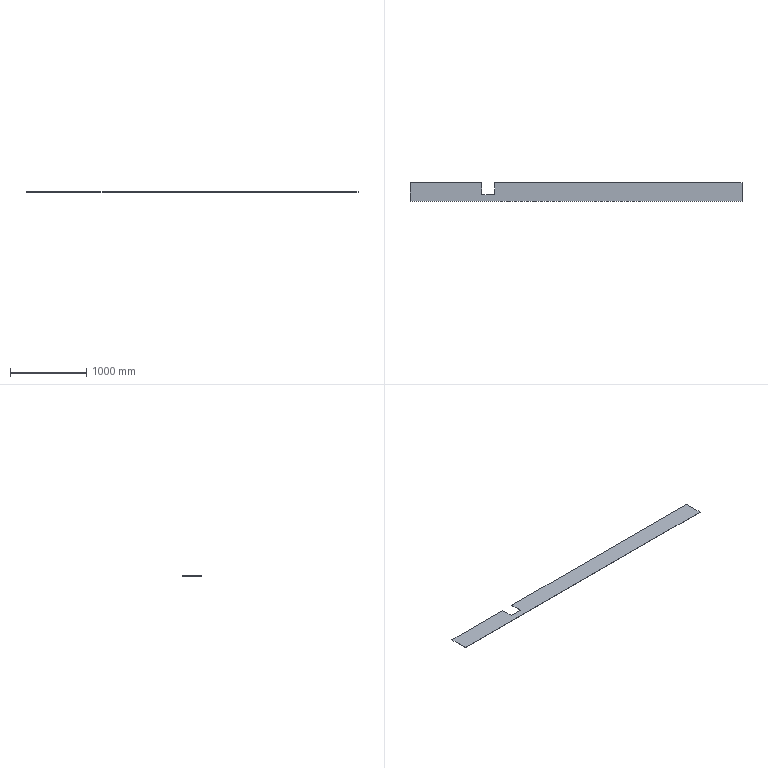Part | STEP file | 休息台花纹Plate 3 | 1 solid | 10 faces | box 4350 x 248 x 3 mm | volume 3156330 mm3 | plane 10
STEP:
#1=CARTESIAN_POINT('',(0.,0.,0.));
#2=DIRECTION('',(0.,0.,1.));
#3=DIRECTION('',(1.,0.,0.));
#4=AXIS2_PLACEMENT_3D('',#1,#2,#3);
#5=CARTESIAN_POINT('',(875.,50.,0.));
#6=VERTEX_POINT('',#5);
#7=CARTESIAN_POINT('',(-2365.,50.,0.));
#8=VERTEX_POINT('',#7);
#9=CARTESIAN_POINT('',(875.,50.,0.));
#10=DIRECTION('',(-1.,0.,0.));
#11=VECTOR('',#10,1.);
#12=LINE('',#9,#11);
#13=CARTESIAN_POINT('',(875.,50.,3.));
#14=DIRECTION('',(0.,-1.,0.));
#15=DIRECTION('',(0.,0.,-1.));
#16=AXIS2_PLACEMENT_3D('',#13,#14,#15);
#17=PLANE('',#16);
#18=CARTESIAN_POINT('',(3.,0.));
#19=DIRECTION('',(0.,-1.));
#20=VECTOR('',#19,1.);
#21=LINE('',#18,#20);
#22=(GEOMETRIC_REPRESENTATION_CONTEXT(2)PARAMETRIC_REPRESENTATION_CONTEXT()REPRESENTATION_CONTEXT('',''));
#23=DEFINITIONAL_REPRESENTATION('',(#21),#22);
#24=PCURVE('',#17,#23);
#25=CARTESIAN_POINT('',(0.,0.,0.));
#26=DIRECTION('',(0.,0.,1.));
#27=DIRECTION('',(1.,0.,0.));
#28=AXIS2_PLACEMENT_3D('',#25,#26,#27);
#29=PLANE('',#28);
#30=CARTESIAN_POINT('',(875.,50.));
#31=DIRECTION('',(-1.,0.));
#32=VECTOR('',#31,1.);
#33=LINE('',#30,#32);
#34=(GEOMETRIC_REPRESENTATION_CONTEXT(2)PARAMETRIC_REPRESENTATION_CONTEXT()REPRESENTATION_CONTEXT('',''));
#35=DEFINITIONAL_REPRESENTATION('',(#33),#34);
#36=PCURVE('',#29,#35);
#37=SURFACE_CURVE('',#12,(#24,#36),.PCURVE_S1.);
#38=EDGE_CURVE('',#6,#8,#37,.T.);
#39=ORIENTED_EDGE('',*,*,#38,.T.);
#40=CARTESIAN_POINT('',(-2365.,50.,3.));
#41=VERTEX_POINT('',#40);
#42=CARTESIAN_POINT('',(-2365.,50.,3.));
#43=DIRECTION('',(0.,0.,-1.));
#44=VECTOR('',#43,1.);
#45=LINE('',#42,#44);
#46=CARTESIAN_POINT('',(0.,-3240.));
#47=DIRECTION('',(1.,0.));
#48=VECTOR('',#47,1.);
#49=LINE('',#46,#48);
#50=(GEOMETRIC_REPRESENTATION_CONTEXT(2)PARAMETRIC_REPRESENTATION_CONTEXT()REPRESENTATION_CONTEXT('',''));
#51=DEFINITIONAL_REPRESENTATION('',(#49),#50);
#52=PCURVE('',#17,#51);
#53=CARTESIAN_POINT('',(-2365.,50.,3.));
#54=DIRECTION('',(1.,0.,0.));
#55=DIRECTION('',(0.,0.,-1.));
#56=AXIS2_PLACEMENT_3D('',#53,#54,#55);
#57=PLANE('',#56);
#58=CARTESIAN_POINT('',(0.,0.));
#59=DIRECTION('',(1.,0.));
#60=VECTOR('',#59,1.);
#61=LINE('',#58,#60);
#62=(GEOMETRIC_REPRESENTATION_CONTEXT(2)PARAMETRIC_REPRESENTATION_CONTEXT()REPRESENTATION_CONTEXT('',''));
#63=DEFINITIONAL_REPRESENTATION('',(#61),#62);
#64=PCURVE('',#57,#63);
#65=SURFACE_CURVE('',#45,(#52,#64),.PCURVE_S1.);
#66=EDGE_CURVE('',#41,#8,#65,.T.);
#67=ORIENTED_EDGE('',*,*,#66,.F.);
#68=CARTESIAN_POINT('',(875.,50.,3.));
#69=VERTEX_POINT('',#68);
#70=CARTESIAN_POINT('',(875.,50.,3.));
#71=DIRECTION('',(-1.,0.,0.));
#72=VECTOR('',#71,1.);
#73=LINE('',#70,#72);
#74=CARTESIAN_POINT('',(0.,0.));
#75=DIRECTION('',(0.,-1.));
#76=VECTOR('',#75,1.);
#77=LINE('',#74,#76);
#78=(GEOMETRIC_REPRESENTATION_CONTEXT(2)PARAMETRIC_REPRESENTATION_CONTEXT()REPRESENTATION_CONTEXT('',''));
#79=DEFINITIONAL_REPRESENTATION('',(#77),#78);
#80=PCURVE('',#17,#79);
#81=CARTESIAN_POINT('',(0.,0.,3.));
#82=DIRECTION('',(0.,0.,1.));
#83=DIRECTION('',(1.,0.,0.));
#84=AXIS2_PLACEMENT_3D('',#81,#82,#83);
#85=PLANE('',#84);
#86=CARTESIAN_POINT('',(875.,50.));
#87=DIRECTION('',(-1.,0.));
#88=VECTOR('',#87,1.);
#89=LINE('',#86,#88);
#90=(GEOMETRIC_REPRESENTATION_CONTEXT(2)PARAMETRIC_REPRESENTATION_CONTEXT()REPRESENTATION_CONTEXT('',''));
#91=DEFINITIONAL_REPRESENTATION('',(#89),#90);
#92=PCURVE('',#85,#91);
#93=SURFACE_CURVE('',#73,(#80,#92),.PCURVE_S1.);
#94=EDGE_CURVE('',#69,#41,#93,.T.);
#95=ORIENTED_EDGE('',*,*,#94,.F.);
#96=CARTESIAN_POINT('',(875.,50.,3.));
#97=DIRECTION('',(0.,0.,-1.));
#98=VECTOR('',#97,1.);
#99=LINE('',#96,#98);
#100=CARTESIAN_POINT('',(0.,0.));
#101=DIRECTION('',(1.,0.));
#102=VECTOR('',#101,1.);
#103=LINE('',#100,#102);
#104=(GEOMETRIC_REPRESENTATION_CONTEXT(2)PARAMETRIC_REPRESENTATION_CONTEXT()REPRESENTATION_CONTEXT('',''));
#105=DEFINITIONAL_REPRESENTATION('',(#103),#104);
#106=PCURVE('',#17,#105);
#107=CARTESIAN_POINT('',(875.,50.,3.));
#108=DIRECTION('',(-1.,0.,0.));
#109=DIRECTION('',(0.,0.,1.));
#110=AXIS2_PLACEMENT_3D('',#107,#108,#109);
#111=PLANE('',#110);
#112=CARTESIAN_POINT('',(0.,0.));
#113=DIRECTION('',(-1.,0.));
#114=VECTOR('',#113,1.);
#115=LINE('',#112,#114);
#116=(GEOMETRIC_REPRESENTATION_CONTEXT(2)PARAMETRIC_REPRESENTATION_CONTEXT()REPRESENTATION_CONTEXT('',''));
#117=DEFINITIONAL_REPRESENTATION('',(#115),#116);
#118=PCURVE('',#111,#117);
#119=SURFACE_CURVE('',#99,(#106,#118),.PCURVE_S1.);
#120=EDGE_CURVE('',#69,#6,#119,.T.);
#121=ORIENTED_EDGE('',*,*,#120,.T.);
#122=EDGE_LOOP('',(#39,#67,#95,#121));
#123=FACE_BOUND('',#122,.T.);
#124=ADVANCED_FACE('',(#123),#17,.F.);
#125=CARTESIAN_POINT('',(-2365.,-107.,0.));
#126=VERTEX_POINT('',#125);
#127=CARTESIAN_POINT('',(-2365.,50.,0.));
#128=DIRECTION('',(0.,-1.,0.));
#129=VECTOR('',#128,1.);
#130=LINE('',#127,#129);
#131=CARTESIAN_POINT('',(3.,0.));
#132=DIRECTION('',(0.,-1.));
#133=VECTOR('',#132,1.);
#134=LINE('',#131,#133);
#135=(GEOMETRIC_REPRESENTATION_CONTEXT(2)PARAMETRIC_REPRESENTATION_CONTEXT()REPRESENTATION_CONTEXT('',''));
#136=DEFINITIONAL_REPRESENTATION('',(#134),#135);
#137=PCURVE('',#57,#136);
#138=CARTESIAN_POINT('',(-2365.,50.));
#139=DIRECTION('',(0.,-1.));
#140=VECTOR('',#139,1.);
#141=LINE('',#138,#140);
#142=(GEOMETRIC_REPRESENTATION_CONTEXT(2)PARAMETRIC_REPRESENTATION_CONTEXT()REPRESENTATION_CONTEXT('',''));
#143=DEFINITIONAL_REPRESENTATION('',(#141),#142);
#144=PCURVE('',#29,#143);
#145=SURFACE_CURVE('',#130,(#137,#144),.PCURVE_S1.);
#146=EDGE_CURVE('',#8,#126,#145,.T.);
#147=ORIENTED_EDGE('',*,*,#146,.T.);
#148=CARTESIAN_POINT('',(-2365.,-107.,3.));
#149=VERTEX_POINT('',#148);
#150=CARTESIAN_POINT('',(-2365.,-107.,3.));
#151=DIRECTION('',(0.,0.,-1.));
#152=VECTOR('',#151,1.);
#153=LINE('',#150,#152);
#154=CARTESIAN_POINT('',(0.,-157.));
#155=DIRECTION('',(1.,0.));
#156=VECTOR('',#155,1.);
#157=LINE('',#154,#156);
#158=(GEOMETRIC_REPRESENTATION_CONTEXT(2)PARAMETRIC_REPRESENTATION_CONTEXT()REPRESENTATION_CONTEXT('',''));
#159=DEFINITIONAL_REPRESENTATION('',(#157),#158);
#160=PCURVE('',#57,#159);
#161=CARTESIAN_POINT('',(-2365.,-107.,3.));
#162=DIRECTION('',(0.,-1.,0.));
#163=DIRECTION('',(1.,0.,0.));
#164=AXIS2_PLACEMENT_3D('',#161,#162,#163);
#165=PLANE('',#164);
#166=CARTESIAN_POINT('',(0.,0.));
#167=DIRECTION('',(0.,-1.));
#168=VECTOR('',#167,1.);
#169=LINE('',#166,#168);
#170=(GEOMETRIC_REPRESENTATION_CONTEXT(2)PARAMETRIC_REPRESENTATION_CONTEXT()REPRESENTATION_CONTEXT('',''));
#171=DEFINITIONAL_REPRESENTATION('',(#169),#170);
#172=PCURVE('',#165,#171);
#173=SURFACE_CURVE('',#153,(#160,#172),.PCURVE_S1.);
#174=EDGE_CURVE('',#149,#126,#173,.T.);
#175=ORIENTED_EDGE('',*,*,#174,.F.);
#176=CARTESIAN_POINT('',(-2365.,50.,3.));
#177=DIRECTION('',(0.,-1.,0.));
#178=VECTOR('',#177,1.);
#179=LINE('',#176,#178);
#180=CARTESIAN_POINT('',(0.,0.));
#181=DIRECTION('',(0.,-1.));
#182=VECTOR('',#181,1.);
#183=LINE('',#180,#182);
#184=(GEOMETRIC_REPRESENTATION_CONTEXT(2)PARAMETRIC_REPRESENTATION_CONTEXT()REPRESENTATION_CONTEXT('',''));
#185=DEFINITIONAL_REPRESENTATION('',(#183),#184);
#186=PCURVE('',#57,#185);
#187=CARTESIAN_POINT('',(-2365.,50.));
#188=DIRECTION('',(0.,-1.));
#189=VECTOR('',#188,1.);
#190=LINE('',#187,#189);
#191=(GEOMETRIC_REPRESENTATION_CONTEXT(2)PARAMETRIC_REPRESENTATION_CONTEXT()REPRESENTATION_CONTEXT('',''));
#192=DEFINITIONAL_REPRESENTATION('',(#190),#191);
#193=PCURVE('',#85,#192);
#194=SURFACE_CURVE('',#179,(#186,#193),.PCURVE_S1.);
#195=EDGE_CURVE('',#41,#149,#194,.T.);
#196=ORIENTED_EDGE('',*,*,#195,.F.);
#197=ORIENTED_EDGE('',*,*,#66,.T.);
#198=EDGE_LOOP('',(#147,#175,#196,#197));
#199=FACE_BOUND('',#198,.T.);
#200=ADVANCED_FACE('',(#199),#57,.F.);
#201=CARTESIAN_POINT('',(-2535.,-107.,0.));
#202=VERTEX_POINT('',#201);
#203=CARTESIAN_POINT('',(-2365.,-107.,0.));
#204=DIRECTION('',(-1.,0.,0.));
#205=VECTOR('',#204,1.);
#206=LINE('',#203,#205);
#207=CARTESIAN_POINT('',(0.,-3.));
#208=DIRECTION('',(-1.,0.));
#209=VECTOR('',#208,1.);
#210=LINE('',#207,#209);
#211=(GEOMETRIC_REPRESENTATION_CONTEXT(2)PARAMETRIC_REPRESENTATION_CONTEXT()REPRESENTATION_CONTEXT('',''));
#212=DEFINITIONAL_REPRESENTATION('',(#210),#211);
#213=PCURVE('',#165,#212);
#214=CARTESIAN_POINT('',(-2365.,-107.));
#215=DIRECTION('',(-1.,0.));
#216=VECTOR('',#215,1.);
#217=LINE('',#214,#216);
#218=(GEOMETRIC_REPRESENTATION_CONTEXT(2)PARAMETRIC_REPRESENTATION_CONTEXT()REPRESENTATION_CONTEXT('',''));
#219=DEFINITIONAL_REPRESENTATION('',(#217),#218);
#220=PCURVE('',#29,#219);
#221=SURFACE_CURVE('',#206,(#213,#220),.PCURVE_S1.);
#222=EDGE_CURVE('',#126,#202,#221,.T.);
#223=ORIENTED_EDGE('',*,*,#222,.T.);
#224=CARTESIAN_POINT('',(-2535.,-107.,3.));
#225=VERTEX_POINT('',#224);
#226=CARTESIAN_POINT('',(-2535.,-107.,3.));
#227=DIRECTION('',(0.,0.,-1.));
#228=VECTOR('',#227,1.);
#229=LINE('',#226,#228);
#230=CARTESIAN_POINT('',(-170.,0.));
#231=DIRECTION('',(0.,-1.));
#232=VECTOR('',#231,1.);
#233=LINE('',#230,#232);
#234=(GEOMETRIC_REPRESENTATION_CONTEXT(2)PARAMETRIC_REPRESENTATION_CONTEXT()REPRESENTATION_CONTEXT('',''));
#235=DEFINITIONAL_REPRESENTATION('',(#233),#234);
#236=PCURVE('',#165,#235);
#237=CARTESIAN_POINT('',(-2535.,50.,3.));
#238=DIRECTION('',(-1.,0.,0.));
#239=DIRECTION('',(0.,0.,1.));
#240=AXIS2_PLACEMENT_3D('',#237,#238,#239);
#241=PLANE('',#240);
#242=CARTESIAN_POINT('',(0.,-157.));
#243=DIRECTION('',(-1.,0.));
#244=VECTOR('',#243,1.);
#245=LINE('',#242,#244);
#246=(GEOMETRIC_REPRESENTATION_CONTEXT(2)PARAMETRIC_REPRESENTATION_CONTEXT()REPRESENTATION_CONTEXT('',''));
#247=DEFINITIONAL_REPRESENTATION('',(#245),#246);
#248=PCURVE('',#241,#247);
#249=SURFACE_CURVE('',#229,(#236,#248),.PCURVE_S1.);
#250=EDGE_CURVE('',#225,#202,#249,.T.);
#251=ORIENTED_EDGE('',*,*,#250,.F.);
#252=CARTESIAN_POINT('',(-2365.,-107.,3.));
#253=DIRECTION('',(-1.,0.,0.));
#254=VECTOR('',#253,1.);
#255=LINE('',#252,#254);
#256=CARTESIAN_POINT('',(0.,0.));
#257=DIRECTION('',(-1.,0.));
#258=VECTOR('',#257,1.);
#259=LINE('',#256,#258);
#260=(GEOMETRIC_REPRESENTATION_CONTEXT(2)PARAMETRIC_REPRESENTATION_CONTEXT()REPRESENTATION_CONTEXT('',''));
#261=DEFINITIONAL_REPRESENTATION('',(#259),#260);
#262=PCURVE('',#165,#261);
#263=CARTESIAN_POINT('',(-2365.,-107.));
#264=DIRECTION('',(-1.,0.));
#265=VECTOR('',#264,1.);
#266=LINE('',#263,#265);
#267=(GEOMETRIC_REPRESENTATION_CONTEXT(2)PARAMETRIC_REPRESENTATION_CONTEXT()REPRESENTATION_CONTEXT('',''));
#268=DEFINITIONAL_REPRESENTATION('',(#266),#267);
#269=PCURVE('',#85,#268);
#270=SURFACE_CURVE('',#255,(#262,#269),.PCURVE_S1.);
#271=EDGE_CURVE('',#149,#225,#270,.T.);
#272=ORIENTED_EDGE('',*,*,#271,.F.);
#273=ORIENTED_EDGE('',*,*,#174,.T.);
#274=EDGE_LOOP('',(#223,#251,#272,#273));
#275=FACE_BOUND('',#274,.T.);
#276=ADVANCED_FACE('',(#275),#165,.F.);
#277=CARTESIAN_POINT('',(-2535.,50.,0.));
#278=VERTEX_POINT('',#277);
#279=CARTESIAN_POINT('',(-2535.,50.,0.));
#280=DIRECTION('',(0.,1.,0.));
#281=VECTOR('',#280,1.);
#282=LINE('',#279,#281);
#283=CARTESIAN_POINT('',(-3.,0.));
#284=DIRECTION('',(0.,1.));
#285=VECTOR('',#284,1.);
#286=LINE('',#283,#285);
#287=(GEOMETRIC_REPRESENTATION_CONTEXT(2)PARAMETRIC_REPRESENTATION_CONTEXT()REPRESENTATION_CONTEXT('',''));
#288=DEFINITIONAL_REPRESENTATION('',(#286),#287);
#289=PCURVE('',#241,#288);
#290=CARTESIAN_POINT('',(-2535.,50.));
#291=DIRECTION('',(0.,1.));
#292=VECTOR('',#291,1.);
#293=LINE('',#290,#292);
#294=(GEOMETRIC_REPRESENTATION_CONTEXT(2)PARAMETRIC_REPRESENTATION_CONTEXT()REPRESENTATION_CONTEXT('',''));
#295=DEFINITIONAL_REPRESENTATION('',(#293),#294);
#296=PCURVE('',#29,#295);
#297=SURFACE_CURVE('',#282,(#289,#296),.PCURVE_S1.);
#298=EDGE_CURVE('',#202,#278,#297,.T.);
#299=ORIENTED_EDGE('',*,*,#298,.T.);
#300=CARTESIAN_POINT('',(-2535.,50.,3.));
#301=VERTEX_POINT('',#300);
#302=CARTESIAN_POINT('',(-2535.,50.,3.));
#303=DIRECTION('',(0.,0.,-1.));
#304=VECTOR('',#303,1.);
#305=LINE('',#302,#304);
#306=CARTESIAN_POINT('',(0.,0.));
#307=DIRECTION('',(-1.,0.));
#308=VECTOR('',#307,1.);
#309=LINE('',#306,#308);
#310=(GEOMETRIC_REPRESENTATION_CONTEXT(2)PARAMETRIC_REPRESENTATION_CONTEXT()REPRESENTATION_CONTEXT('',''));
#311=DEFINITIONAL_REPRESENTATION('',(#309),#310);
#312=PCURVE('',#241,#311);
#313=CARTESIAN_POINT('',(-2535.,50.,3.));
#314=DIRECTION('',(0.,-1.,0.));
#315=DIRECTION('',(1.,0.,0.));
#316=AXIS2_PLACEMENT_3D('',#313,#314,#315);
#317=PLANE('',#316);
#318=CARTESIAN_POINT('',(0.,0.));
#319=DIRECTION('',(0.,-1.));
#320=VECTOR('',#319,1.);
#321=LINE('',#318,#320);
#322=(GEOMETRIC_REPRESENTATION_CONTEXT(2)PARAMETRIC_REPRESENTATION_CONTEXT()REPRESENTATION_CONTEXT('',''));
#323=DEFINITIONAL_REPRESENTATION('',(#321),#322);
#324=PCURVE('',#317,#323);
#325=SURFACE_CURVE('',#305,(#312,#324),.PCURVE_S1.);
#326=EDGE_CURVE('',#301,#278,#325,.T.);
#327=ORIENTED_EDGE('',*,*,#326,.F.);
#328=CARTESIAN_POINT('',(-2535.,50.,3.));
#329=DIRECTION('',(0.,1.,0.));
#330=VECTOR('',#329,1.);
#331=LINE('',#328,#330);
#332=CARTESIAN_POINT('',(0.,0.));
#333=DIRECTION('',(0.,1.));
#334=VECTOR('',#333,1.);
#335=LINE('',#332,#334);
#336=(GEOMETRIC_REPRESENTATION_CONTEXT(2)PARAMETRIC_REPRESENTATION_CONTEXT()REPRESENTATION_CONTEXT('',''));
#337=DEFINITIONAL_REPRESENTATION('',(#335),#336);
#338=PCURVE('',#241,#337);
#339=CARTESIAN_POINT('',(-2535.,50.));
#340=DIRECTION('',(0.,1.));
#341=VECTOR('',#340,1.);
#342=LINE('',#339,#341);
#343=(GEOMETRIC_REPRESENTATION_CONTEXT(2)PARAMETRIC_REPRESENTATION_CONTEXT()REPRESENTATION_CONTEXT('',''));
#344=DEFINITIONAL_REPRESENTATION('',(#342),#343);
#345=PCURVE('',#85,#344);
#346=SURFACE_CURVE('',#331,(#338,#345),.PCURVE_S1.);
#347=EDGE_CURVE('',#225,#301,#346,.T.);
#348=ORIENTED_EDGE('',*,*,#347,.F.);
#349=ORIENTED_EDGE('',*,*,#250,.T.);
#350=EDGE_LOOP('',(#299,#327,#348,#349));
#351=FACE_BOUND('',#350,.T.);
#352=ADVANCED_FACE('',(#351),#241,.F.);
#353=CARTESIAN_POINT('',(-3475.,50.,0.));
#354=VERTEX_POINT('',#353);
#355=CARTESIAN_POINT('',(-2535.,50.,0.));
#356=DIRECTION('',(-1.,0.,0.));
#357=VECTOR('',#356,1.);
#358=LINE('',#355,#357);
#359=CARTESIAN_POINT('',(0.,-3.));
#360=DIRECTION('',(-1.,0.));
#361=VECTOR('',#360,1.);
#362=LINE('',#359,#361);
#363=(GEOMETRIC_REPRESENTATION_CONTEXT(2)PARAMETRIC_REPRESENTATION_CONTEXT()REPRESENTATION_CONTEXT('',''));
#364=DEFINITIONAL_REPRESENTATION('',(#362),#363);
#365=PCURVE('',#317,#364);
#366=CARTESIAN_POINT('',(-2535.,50.));
#367=DIRECTION('',(-1.,0.));
#368=VECTOR('',#367,1.);
#369=LINE('',#366,#368);
#370=(GEOMETRIC_REPRESENTATION_CONTEXT(2)PARAMETRIC_REPRESENTATION_CONTEXT()REPRESENTATION_CONTEXT('',''));
#371=DEFINITIONAL_REPRESENTATION('',(#369),#370);
#372=PCURVE('',#29,#371);
#373=SURFACE_CURVE('',#358,(#365,#372),.PCURVE_S1.);
#374=EDGE_CURVE('',#278,#354,#373,.T.);
#375=ORIENTED_EDGE('',*,*,#374,.T.);
#376=CARTESIAN_POINT('',(-3475.,50.,3.));
#377=VERTEX_POINT('',#376);
#378=CARTESIAN_POINT('',(-3475.,50.,3.));
#379=DIRECTION('',(0.,0.,-1.));
#380=VECTOR('',#379,1.);
#381=LINE('',#378,#380);
#382=CARTESIAN_POINT('',(-940.,0.));
#383=DIRECTION('',(0.,-1.));
#384=VECTOR('',#383,1.);
#385=LINE('',#382,#384);
#386=(GEOMETRIC_REPRESENTATION_CONTEXT(2)PARAMETRIC_REPRESENTATION_CONTEXT()REPRESENTATION_CONTEXT('',''));
#387=DEFINITIONAL_REPRESENTATION('',(#385),#386);
#388=PCURVE('',#317,#387);
#389=CARTESIAN_POINT('',(-3475.,50.,3.));
#390=DIRECTION('',(1.,0.,0.));
#391=DIRECTION('',(0.,0.,-1.));
#392=AXIS2_PLACEMENT_3D('',#389,#390,#391);
#393=PLANE('',#392);
#394=CARTESIAN_POINT('',(0.,0.));
#395=DIRECTION('',(1.,0.));
#396=VECTOR('',#395,1.);
#397=LINE('',#394,#396);
#398=(GEOMETRIC_REPRESENTATION_CONTEXT(2)PARAMETRIC_REPRESENTATION_CONTEXT()REPRESENTATION_CONTEXT('',''));
#399=DEFINITIONAL_REPRESENTATION('',(#397),#398);
#400=PCURVE('',#393,#399);
#401=SURFACE_CURVE('',#381,(#388,#400),.PCURVE_S1.);
#402=EDGE_CURVE('',#377,#354,#401,.T.);
#403=ORIENTED_EDGE('',*,*,#402,.F.);
#404=CARTESIAN_POINT('',(-2535.,50.,3.));
#405=DIRECTION('',(-1.,0.,0.));
#406=VECTOR('',#405,1.);
#407=LINE('',#404,#406);
#408=CARTESIAN_POINT('',(0.,0.));
#409=DIRECTION('',(-1.,0.));
#410=VECTOR('',#409,1.);
#411=LINE('',#408,#410);
#412=(GEOMETRIC_REPRESENTATION_CONTEXT(2)PARAMETRIC_REPRESENTATION_CONTEXT()REPRESENTATION_CONTEXT('',''));
#413=DEFINITIONAL_REPRESENTATION('',(#411),#412);
#414=PCURVE('',#317,#413);
#415=CARTESIAN_POINT('',(-2535.,50.));
#416=DIRECTION('',(-1.,0.));
#417=VECTOR('',#416,1.);
#418=LINE('',#415,#417);
#419=(GEOMETRIC_REPRESENTATION_CONTEXT(2)PARAMETRIC_REPRESENTATION_CONTEXT()REPRESENTATION_CONTEXT('',''));
#420=DEFINITIONAL_REPRESENTATION('',(#418),#419);
#421=PCURVE('',#85,#420);
#422=SURFACE_CURVE('',#407,(#414,#421),.PCURVE_S1.);
#423=EDGE_CURVE('',#301,#377,#422,.T.);
#424=ORIENTED_EDGE('',*,*,#423,.F.);
#425=ORIENTED_EDGE('',*,*,#326,.T.);
#426=EDGE_LOOP('',(#375,#403,#424,#425));
#427=FACE_BOUND('',#426,.T.);
#428=ADVANCED_FACE('',(#427),#317,.F.);
#429=CARTESIAN_POINT('',(-3475.,-198.,0.));
#430=VERTEX_POINT('',#429);
#431=CARTESIAN_POINT('',(-3475.,50.,0.));
#432=DIRECTION('',(0.,-1.,0.));
#433=VECTOR('',#432,1.);
#434=LINE('',#431,#433);
#435=CARTESIAN_POINT('',(3.,0.));
#436=DIRECTION('',(0.,-1.));
#437=VECTOR('',#436,1.);
#438=LINE('',#435,#437);
#439=(GEOMETRIC_REPRESENTATION_CONTEXT(2)PARAMETRIC_REPRESENTATION_CONTEXT()REPRESENTATION_CONTEXT('',''));
#440=DEFINITIONAL_REPRESENTATION('',(#438),#439);
#441=PCURVE('',#393,#440);
#442=CARTESIAN_POINT('',(-3475.,50.));
#443=DIRECTION('',(0.,-1.));
#444=VECTOR('',#443,1.);
#445=LINE('',#442,#444);
#446=(GEOMETRIC_REPRESENTATION_CONTEXT(2)PARAMETRIC_REPRESENTATION_CONTEXT()REPRESENTATION_CONTEXT('',''));
#447=DEFINITIONAL_REPRESENTATION('',(#445),#446);
#448=PCURVE('',#29,#447);
#449=SURFACE_CURVE('',#434,(#441,#448),.PCURVE_S1.);
#450=EDGE_CURVE('',#354,#430,#449,.T.);
#451=ORIENTED_EDGE('',*,*,#450,.T.);
#452=CARTESIAN_POINT('',(-3475.,-198.,3.));
#453=VERTEX_POINT('',#452);
#454=CARTESIAN_POINT('',(-3475.,-198.,3.));
#455=DIRECTION('',(0.,0.,-1.));
#456=VECTOR('',#455,1.);
#457=LINE('',#454,#456);
#458=CARTESIAN_POINT('',(0.,-248.));
#459=DIRECTION('',(1.,0.));
#460=VECTOR('',#459,1.);
#461=LINE('',#458,#460);
#462=(GEOMETRIC_REPRESENTATION_CONTEXT(2)PARAMETRIC_REPRESENTATION_CONTEXT()REPRESENTATION_CONTEXT('',''));
#463=DEFINITIONAL_REPRESENTATION('',(#461),#462);
#464=PCURVE('',#393,#463);
#465=CARTESIAN_POINT('',(875.,-198.,3.));
#466=DIRECTION('',(0.,1.,0.));
#467=DIRECTION('',(-1.,0.,0.));
#468=AXIS2_PLACEMENT_3D('',#465,#466,#467);
#469=PLANE('',#468);
#470=CARTESIAN_POINT('',(4350.,0.));
#471=DIRECTION('',(0.,-1.));
#472=VECTOR('',#471,1.);
#473=LINE('',#470,#472);
#474=(GEOMETRIC_REPRESENTATION_CONTEXT(2)PARAMETRIC_REPRESENTATION_CONTEXT()REPRESENTATION_CONTEXT('',''));
#475=DEFINITIONAL_REPRESENTATION('',(#473),#474);
#476=PCURVE('',#469,#475);
#477=SURFACE_CURVE('',#457,(#464,#476),.PCURVE_S1.);
#478=EDGE_CURVE('',#453,#430,#477,.T.);
#479=ORIENTED_EDGE('',*,*,#478,.F.);
#480=CARTESIAN_POINT('',(-3475.,50.,3.));
#481=DIRECTION('',(0.,-1.,0.));
#482=VECTOR('',#481,1.);
#483=LINE('',#480,#482);
#484=CARTESIAN_POINT('',(0.,0.));
#485=DIRECTION('',(0.,-1.));
#486=VECTOR('',#485,1.);
#487=LINE('',#484,#486);
#488=(GEOMETRIC_REPRESENTATION_CONTEXT(2)PARAMETRIC_REPRESENTATION_CONTEXT()REPRESENTATION_CONTEXT('',''));
#489=DEFINITIONAL_REPRESENTATION('',(#487),#488);
#490=PCURVE('',#393,#489);
#491=CARTESIAN_POINT('',(-3475.,50.));
#492=DIRECTION('',(0.,-1.));
#493=VECTOR('',#492,1.);
#494=LINE('',#491,#493);
#495=(GEOMETRIC_REPRESENTATION_CONTEXT(2)PARAMETRIC_REPRESENTATION_CONTEXT()REPRESENTATION_CONTEXT('',''));
#496=DEFINITIONAL_REPRESENTATION('',(#494),#495);
#497=PCURVE('',#85,#496);
#498=SURFACE_CURVE('',#483,(#490,#497),.PCURVE_S1.);
#499=EDGE_CURVE('',#377,#453,#498,.T.);
#500=ORIENTED_EDGE('',*,*,#499,.F.);
#501=ORIENTED_EDGE('',*,*,#402,.T.);
#502=EDGE_LOOP('',(#451,#479,#500,#501));
#503=FACE_BOUND('',#502,.T.);
#504=ADVANCED_FACE('',(#503),#393,.F.);
#505=CARTESIAN_POINT('',(875.,-198.,0.));
#506=VERTEX_POINT('',#505);
#507=CARTESIAN_POINT('',(875.,-198.,0.));
#508=DIRECTION('',(1.,0.,0.));
#509=VECTOR('',#508,1.);
#510=LINE('',#507,#509);
#511=CARTESIAN_POINT('',(0.,-3.));
#512=DIRECTION('',(-1.,0.));
#513=VECTOR('',#512,1.);
#514=LINE('',#511,#513);
#515=(GEOMETRIC_REPRESENTATION_CONTEXT(2)PARAMETRIC_REPRESENTATION_CONTEXT()REPRESENTATION_CONTEXT('',''));
#516=DEFINITIONAL_REPRESENTATION('',(#514),#515);
#517=PCURVE('',#469,#516);
#518=CARTESIAN_POINT('',(875.,-198.));
#519=DIRECTION('',(1.,0.));
#520=VECTOR('',#519,1.);
#521=LINE('',#518,#520);
#522=(GEOMETRIC_REPRESENTATION_CONTEXT(2)PARAMETRIC_REPRESENTATION_CONTEXT()REPRESENTATION_CONTEXT('',''));
#523=DEFINITIONAL_REPRESENTATION('',(#521),#522);
#524=PCURVE('',#29,#523);
#525=SURFACE_CURVE('',#510,(#517,#524),.PCURVE_S1.);
#526=EDGE_CURVE('',#430,#506,#525,.T.);
#527=ORIENTED_EDGE('',*,*,#526,.T.);
#528=CARTESIAN_POINT('',(875.,-198.,3.));
#529=VERTEX_POINT('',#528);
#530=CARTESIAN_POINT('',(875.,-198.,3.));
#531=DIRECTION('',(0.,0.,-1.));
#532=VECTOR('',#531,1.);
#533=LINE('',#530,#532);
#534=CARTESIAN_POINT('',(0.,0.));
#535=DIRECTION('',(0.,-1.));
#536=VECTOR('',#535,1.);
#537=LINE('',#534,#536);
#538=(GEOMETRIC_REPRESENTATION_CONTEXT(2)PARAMETRIC_REPRESENTATION_CONTEXT()REPRESENTATION_CONTEXT('',''));
#539=DEFINITIONAL_REPRESENTATION('',(#537),#538);
#540=PCURVE('',#469,#539);
#541=CARTESIAN_POINT('',(0.,-248.));
#542=DIRECTION('',(-1.,0.));
#543=VECTOR('',#542,1.);
#544=LINE('',#541,#543);
#545=(GEOMETRIC_REPRESENTATION_CONTEXT(2)PARAMETRIC_REPRESENTATION_CONTEXT()REPRESENTATION_CONTEXT('',''));
#546=DEFINITIONAL_REPRESENTATION('',(#544),#545);
#547=PCURVE('',#111,#546);
#548=SURFACE_CURVE('',#533,(#540,#547),.PCURVE_S1.);
#549=EDGE_CURVE('',#529,#506,#548,.T.);
#550=ORIENTED_EDGE('',*,*,#549,.F.);
#551=CARTESIAN_POINT('',(875.,-198.,3.));
#552=DIRECTION('',(1.,0.,0.));
#553=VECTOR('',#552,1.);
#554=LINE('',#551,#553);
#555=CARTESIAN_POINT('',(0.,0.));
#556=DIRECTION('',(-1.,0.));
#557=VECTOR('',#556,1.);
#558=LINE('',#555,#557);
#559=(GEOMETRIC_REPRESENTATION_CONTEXT(2)PARAMETRIC_REPRESENTATION_CONTEXT()REPRESENTATION_CONTEXT('',''));
#560=DEFINITIONAL_REPRESENTATION('',(#558),#559);
#561=PCURVE('',#469,#560);
#562=CARTESIAN_POINT('',(875.,-198.));
#563=DIRECTION('',(1.,0.));
#564=VECTOR('',#563,1.);
#565=LINE('',#562,#564);
#566=(GEOMETRIC_REPRESENTATION_CONTEXT(2)PARAMETRIC_REPRESENTATION_CONTEXT()REPRESENTATION_CONTEXT('',''));
#567=DEFINITIONAL_REPRESENTATION('',(#565),#566);
#568=PCURVE('',#85,#567);
#569=SURFACE_CURVE('',#554,(#561,#568),.PCURVE_S1.);
#570=EDGE_CURVE('',#453,#529,#569,.T.);
#571=ORIENTED_EDGE('',*,*,#570,.F.);
#572=ORIENTED_EDGE('',*,*,#478,.T.);
#573=EDGE_LOOP('',(#527,#550,#571,#572));
#574=FACE_BOUND('',#573,.T.);
#575=ADVANCED_FACE('',(#574),#469,.F.);
#576=CARTESIAN_POINT('',(875.,50.,0.));
#577=DIRECTION('',(0.,1.,0.));
#578=VECTOR('',#577,1.);
#579=LINE('',#576,#578);
#580=CARTESIAN_POINT('',(-3.,0.));
#581=DIRECTION('',(0.,1.));
#582=VECTOR('',#581,1.);
#583=LINE('',#580,#582);
#584=(GEOMETRIC_REPRESENTATION_CONTEXT(2)PARAMETRIC_REPRESENTATION_CONTEXT()REPRESENTATION_CONTEXT('',''));
#585=DEFINITIONAL_REPRESENTATION('',(#583),#584);
#586=PCURVE('',#111,#585);
#587=CARTESIAN_POINT('',(875.,50.));
#588=DIRECTION('',(0.,1.));
#589=VECTOR('',#588,1.);
#590=LINE('',#587,#589);
#591=(GEOMETRIC_REPRESENTATION_CONTEXT(2)PARAMETRIC_REPRESENTATION_CONTEXT()REPRESENTATION_CONTEXT('',''));
#592=DEFINITIONAL_REPRESENTATION('',(#590),#591);
#593=PCURVE('',#29,#592);
#594=SURFACE_CURVE('',#579,(#586,#593),.PCURVE_S1.);
#595=EDGE_CURVE('',#506,#6,#594,.T.);
#596=ORIENTED_EDGE('',*,*,#595,.T.);
#597=ORIENTED_EDGE('',*,*,#120,.F.);
#598=CARTESIAN_POINT('',(875.,50.,3.));
#599=DIRECTION('',(0.,1.,0.));
#600=VECTOR('',#599,1.);
#601=LINE('',#598,#600);
#602=CARTESIAN_POINT('',(0.,0.));
#603=DIRECTION('',(0.,1.));
#604=VECTOR('',#603,1.);
#605=LINE('',#602,#604);
#606=(GEOMETRIC_REPRESENTATION_CONTEXT(2)PARAMETRIC_REPRESENTATION_CONTEXT()REPRESENTATION_CONTEXT('',''));
#607=DEFINITIONAL_REPRESENTATION('',(#605),#606);
#608=PCURVE('',#111,#607);
#609=CARTESIAN_POINT('',(875.,50.));
#610=DIRECTION('',(0.,1.));
#611=VECTOR('',#610,1.);
#612=LINE('',#609,#611);
#613=(GEOMETRIC_REPRESENTATION_CONTEXT(2)PARAMETRIC_REPRESENTATION_CONTEXT()REPRESENTATION_CONTEXT('',''));
#614=DEFINITIONAL_REPRESENTATION('',(#612),#613);
#615=PCURVE('',#85,#614);
#616=SURFACE_CURVE('',#601,(#608,#615),.PCURVE_S1.);
#617=EDGE_CURVE('',#529,#69,#616,.T.);
#618=ORIENTED_EDGE('',*,*,#617,.F.);
#619=ORIENTED_EDGE('',*,*,#549,.T.);
#620=EDGE_LOOP('',(#596,#597,#618,#619));
#621=FACE_BOUND('',#620,.T.);
#622=ADVANCED_FACE('',(#621),#111,.F.);
#623=ORIENTED_EDGE('',*,*,#94,.T.);
#624=ORIENTED_EDGE('',*,*,#195,.T.);
#625=ORIENTED_EDGE('',*,*,#271,.T.);
#626=ORIENTED_EDGE('',*,*,#347,.T.);
#627=ORIENTED_EDGE('',*,*,#423,.T.);
#628=ORIENTED_EDGE('',*,*,#499,.T.);
#629=ORIENTED_EDGE('',*,*,#570,.T.);
#630=ORIENTED_EDGE('',*,*,#617,.T.);
#631=EDGE_LOOP('',(#623,#624,#625,#626,#627,#628,#629,#630));
#632=FACE_BOUND('',#631,.T.);
#633=ADVANCED_FACE('',(#632),#85,.T.);
#634=ORIENTED_EDGE('',*,*,#38,.F.);
#635=ORIENTED_EDGE('',*,*,#595,.F.);
#636=ORIENTED_EDGE('',*,*,#526,.F.);
#637=ORIENTED_EDGE('',*,*,#450,.F.);
#638=ORIENTED_EDGE('',*,*,#374,.F.);
#639=ORIENTED_EDGE('',*,*,#298,.F.);
#640=ORIENTED_EDGE('',*,*,#222,.F.);
#641=ORIENTED_EDGE('',*,*,#146,.F.);
#642=EDGE_LOOP('',(#634,#635,#636,#637,#638,#639,#640,#641));
#643=FACE_BOUND('',#642,.T.);
#644=ADVANCED_FACE('',(#643),#29,.F.);
#645=CLOSED_SHELL('',(#124,#200,#276,#352,#428,#504,#575,#622,#633,#644));
#646=MANIFOLD_SOLID_BREP('',#645);
#647=(LENGTH_UNIT()NAMED_UNIT(*)SI_UNIT(.MILLI.,.METRE.));
#648=UNCERTAINTY_MEASURE_WITH_UNIT(LENGTH_MEASURE(0.0000001),#647,'','');
#649=(NAMED_UNIT(*)PLANE_ANGLE_UNIT()SI_UNIT($,.RADIAN.));
#650=(NAMED_UNIT(*)SI_UNIT($,.STERADIAN.)SOLID_ANGLE_UNIT());
#651=(GEOMETRIC_REPRESENTATION_CONTEXT(3)GLOBAL_UNCERTAINTY_ASSIGNED_CONTEXT((#648))GLOBAL_UNIT_ASSIGNED_CONTEXT((#647,#649,#650))REPRESENTATION_CONTEXT('',''));
#652=ADVANCED_BREP_SHAPE_REPRESENTATION('',(#4,#646),#651);